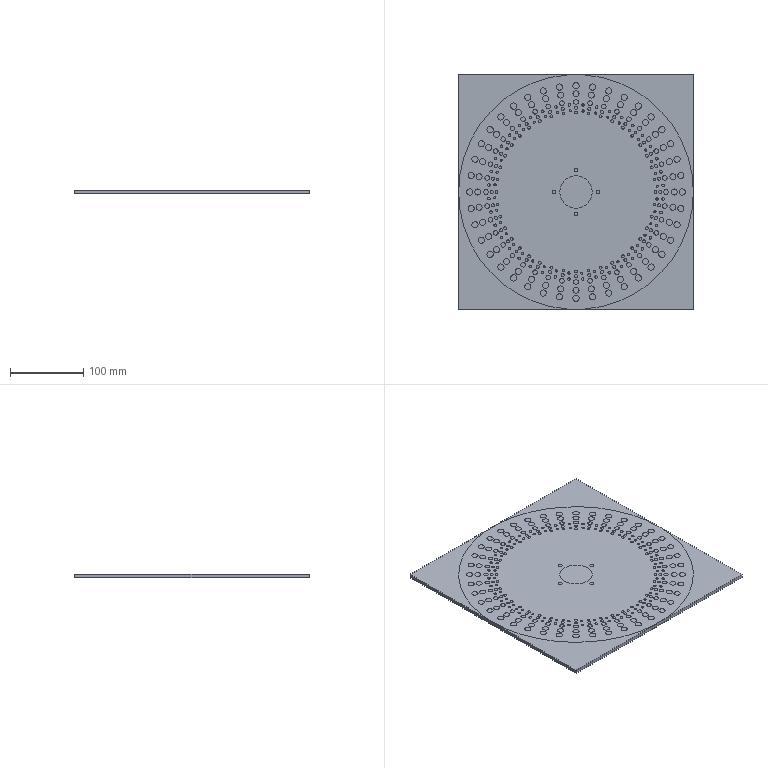NC program | NX | posted with a generic post | part box 320 x 320 x 5 mm
Lines 39666 to 40337 of 63198:
(孔铣精光G41 , TOOL : D6平底刀)
N79324 T08 M6
N79326 /M1
N79328 G54
N79330 G17 G0 G90 X0. Y144.747 S3000 M3
N79332 G43 Z20. H8
N79334 Z1.2
N79336 G94 G1 Z0.2 F400.
N79338 G41 X0.01 Y144.647 D8
N79340 G3 X2.025 Y144.747 R1.01
N79342 X2.025 Y144.747 Z0. I-2.025 J0. F500.
N79344 X2.025 Y144.747 Z-0.2 I-2.025 J0.
N79346 X2.025 Y144.747 Z-0.4 I-2.025 J0.
N79348 X2.025 Y144.747 Z-0.6 I-2.025 J0.
N79350 X2.025 Y144.747 Z-0.8 I-2.025 J0.
N79352 X2.025 Y144.747 Z-1. I-2.025 J0.
N79354 X2.025 Y144.747 Z-1.2 I-2.025 J0.
N79356 X2.025 Y144.747 Z-1.4 I-2.025 J0.
N79358 X2.025 Y144.747 Z-1.6 I-2.025 J0.
N79360 X2.025 Y144.747 Z-1.8 I-2.025 J0.
N79362 X2.025 Y144.747 Z-2. I-2.025 J0.
N79364 X2.025 Y144.747 Z-2.2 I-2.025 J0.
N79366 X2.025 Y144.747 Z-2.4 I-2.025 J0.
N79368 X2.025 Y144.747 Z-2.6 I-2.025 J0.
N79370 X2.025 Y144.747 Z-2.8 I-2.025 J0.
N79372 X2.025 Y144.747 Z-3. I-2.025 J0.
N79374 X2.025 Y144.747 Z-3.2 I-2.025 J0.
N79376 X2.025 Y144.747 Z-3.4 I-2.025 J0.
N79378 X2.025 Y144.747 Z-3.6 I-2.025 J0.
N79380 X2.025 Y144.747 Z-3.8 I-2.025 J0.
N79382 X2.025 Y144.747 Z-4. I-2.025 J0.
N79384 X2.025 Y144.747 Z-4.2 I-2.025 J0.
N79386 X2.025 Y144.747 Z-4.4 I-2.025 J0.
N79388 X2.025 Y144.747 Z-4.6 I-2.025 J0.
N79390 X2.025 Y144.747 Z-4.8 I-2.025 J0.
N79392 X2.025 Y144.747 Z-5. I-2.025 J0.
N79394 X0. Y146.772 R2.025
N79396 X2.025 Y144.747 R-2.025
N79398 X0.01 Y144.846 R1.01
N79400 G40
N79402 G1 X0. Y144.747
N79404 Z-4.8
N79406 G0 Z20.
N79408 X22.643 Y142.965
N79410 Z1.2
N79412 G1 Z0.2 F400.
N79414 G41 X22.653 Y142.865
N79416 G3 X24.668 Y142.965 R1.01
N79418 X24.668 Y142.965 Z0. I-2.025 J0. F500.
N79420 X24.668 Y142.965 Z-0.2 I-2.025 J0.
N79422 X24.668 Y142.965 Z-0.4 I-2.025 J0.
N79424 X24.668 Y142.965 Z-0.6 I-2.025 J0.
N79426 X24.668 Y142.965 Z-0.8 I-2.025 J0.
N79428 X24.668 Y142.965 Z-1. I-2.025 J0.
N79430 X24.668 Y142.965 Z-1.2 I-2.025 J0.
N79432 X24.668 Y142.965 Z-1.4 I-2.025 J0.
N79434 X24.668 Y142.965 Z-1.6 I-2.025 J0.
N79436 X24.668 Y142.965 Z-1.8 I-2.025 J0.
N79438 X24.668 Y142.965 Z-2. I-2.025 J0.
N79440 X24.668 Y142.965 Z-2.2 I-2.025 J0.
N79442 X24.668 Y142.965 Z-2.4 I-2.025 J0.
N79444 X24.668 Y142.965 Z-2.6 I-2.025 J0.
N79446 X24.668 Y142.965 Z-2.8 I-2.025 J0.
N79448 X24.668 Y142.965 Z-3. I-2.025 J0.
N79450 X24.668 Y142.965 Z-3.2 I-2.025 J0.
N79452 X24.668 Y142.965 Z-3.4 I-2.025 J0.
N79454 X24.668 Y142.965 Z-3.6 I-2.025 J0.
N79456 X24.668 Y142.965 Z-3.8 I-2.025 J0.
N79458 X24.668 Y142.965 Z-4. I-2.025 J0.
N79460 X24.668 Y142.965 Z-4.2 I-2.025 J0.
N79462 X24.668 Y142.965 Z-4.4 I-2.025 J0.
N79464 X24.668 Y142.965 Z-4.6 I-2.025 J0.
N79466 X24.668 Y142.965 Z-4.8 I-2.025 J0.
N79468 X24.668 Y142.965 Z-5. I-2.025 J0.
N79470 X22.643 Y144.99 R2.025
N79472 X24.668 Y142.965 R-2.025
N79474 X22.653 Y143.064 R1.01
N79476 G40
N79478 G1 X22.643 Y142.965
N79480 Z-4.8
N79482 G0 Z20.
N79484 X44.729 Y137.662
N79486 Z1.2
N79488 G1 Z0.2 F400.
N79490 G41 X44.739 Y137.563
N79492 G3 X46.754 Y137.662 R1.01
N79494 X46.754 Y137.662 Z0. I-2.025 J0. F500.
N79496 X46.754 Y137.662 Z-0.2 I-2.025 J0.
N79498 X46.754 Y137.662 Z-0.4 I-2.025 J0.
N79500 X46.754 Y137.662 Z-0.6 I-2.025 J0.
N79502 X46.754 Y137.662 Z-0.8 I-2.025 J0.
N79504 X46.754 Y137.662 Z-1. I-2.025 J0.
N79506 X46.754 Y137.662 Z-1.2 I-2.025 J0.
N79508 X46.754 Y137.662 Z-1.4 I-2.025 J0.
N79510 X46.754 Y137.662 Z-1.6 I-2.025 J0.
N79512 X46.754 Y137.662 Z-1.8 I-2.025 J0.
N79514 X46.754 Y137.662 Z-2. I-2.025 J0.
N79516 X46.754 Y137.662 Z-2.2 I-2.025 J0.
N79518 X46.754 Y137.662 Z-2.4 I-2.025 J0.
N79520 X46.754 Y137.662 Z-2.6 I-2.025 J0.
N79522 X46.754 Y137.662 Z-2.8 I-2.025 J0.
N79524 X46.754 Y137.662 Z-3. I-2.025 J0.
N79526 X46.754 Y137.662 Z-3.2 I-2.025 J0.
N79528 X46.754 Y137.662 Z-3.4 I-2.025 J0.
N79530 X46.754 Y137.662 Z-3.6 I-2.025 J0.
N79532 X46.754 Y137.662 Z-3.8 I-2.025 J0.
N79534 X46.754 Y137.662 Z-4. I-2.025 J0.
N79536 X46.754 Y137.662 Z-4.2 I-2.025 J0.
N79538 X46.754 Y137.662 Z-4.4 I-2.025 J0.
N79540 X46.754 Y137.662 Z-4.6 I-2.025 J0.
N79542 X46.754 Y137.662 Z-4.8 I-2.025 J0.
N79544 X46.754 Y137.662 Z-5. I-2.025 J0.
N79546 X44.729 Y139.687 R2.025
N79548 X46.754 Y137.662 R-2.025
N79550 X44.739 Y137.762 R1.01
N79552 G40
N79554 G1 X44.729 Y137.662
N79556 Z-4.8
N79558 G0 Z20.
N79560 X65.714 Y128.97
N79562 Z1.2
N79564 G1 Z0.2 F400.
N79566 G41 X65.724 Y128.871
N79568 G3 X67.739 Y128.97 R1.01
N79570 X67.739 Y128.97 Z0. I-2.025 J0. F500.
N79572 X67.739 Y128.97 Z-0.2 I-2.025 J0.
N79574 X67.739 Y128.97 Z-0.4 I-2.025 J0.
N79576 X67.739 Y128.97 Z-0.6 I-2.025 J0.
N79578 X67.739 Y128.97 Z-0.8 I-2.025 J0.
N79580 X67.739 Y128.97 Z-1. I-2.025 J0.
N79582 X67.739 Y128.97 Z-1.2 I-2.025 J0.
N79584 X67.739 Y128.97 Z-1.4 I-2.025 J0.
N79586 X67.739 Y128.97 Z-1.6 I-2.025 J0.
N79588 X67.739 Y128.97 Z-1.8 I-2.025 J0.
N79590 X67.739 Y128.97 Z-2. I-2.025 J0.
N79592 X67.739 Y128.97 Z-2.2 I-2.025 J0.
N79594 X67.739 Y128.97 Z-2.4 I-2.025 J0.
N79596 X67.739 Y128.97 Z-2.6 I-2.025 J0.
N79598 X67.739 Y128.97 Z-2.8 I-2.025 J0.
N79600 X67.739 Y128.97 Z-3. I-2.025 J0.
N79602 X67.739 Y128.97 Z-3.2 I-2.025 J0.
N79604 X67.739 Y128.97 Z-3.4 I-2.025 J0.
N79606 X67.739 Y128.97 Z-3.6 I-2.025 J0.
N79608 X67.739 Y128.97 Z-3.8 I-2.025 J0.
N79610 X67.739 Y128.97 Z-4. I-2.025 J0.
N79612 X67.739 Y128.97 Z-4.2 I-2.025 J0.
N79614 X67.739 Y128.97 Z-4.4 I-2.025 J0.
N79616 X67.739 Y128.97 Z-4.6 I-2.025 J0.
N79618 X67.739 Y128.97 Z-4.8 I-2.025 J0.
N79620 X67.739 Y128.97 Z-5. I-2.025 J0.
N79622 X65.714 Y130.995 R2.025
N79624 X67.739 Y128.97 R-2.025
N79626 X65.724 Y129.07 R1.01
N79628 G40
N79630 G1 X65.714 Y128.97
N79632 Z-4.8
N79634 G0 Z20.
N79636 X85.08 Y117.103
N79638 Z1.2
N79640 G1 Z0.2 F400.
N79642 G41 X85.09 Y117.003
N79644 G3 X87.105 Y117.103 R1.01
N79646 X87.105 Y117.103 Z0. I-2.025 J0. F500.
N79648 X87.105 Y117.103 Z-0.2 I-2.025 J0.
N79650 X87.105 Y117.103 Z-0.4 I-2.025 J0.
N79652 X87.105 Y117.103 Z-0.6 I-2.025 J0.
N79654 X87.105 Y117.103 Z-0.8 I-2.025 J0.
N79656 X87.105 Y117.103 Z-1. I-2.025 J0.
N79658 X87.105 Y117.103 Z-1.2 I-2.025 J0.
N79660 X87.105 Y117.103 Z-1.4 I-2.025 J0.
N79662 X87.105 Y117.103 Z-1.6 I-2.025 J0.
N79664 X87.105 Y117.103 Z-1.8 I-2.025 J0.
N79666 X87.105 Y117.103 Z-2. I-2.025 J0.
N79668 X87.105 Y117.103 Z-2.2 I-2.025 J0.
N79670 X87.105 Y117.103 Z-2.4 I-2.025 J0.
N79672 X87.105 Y117.103 Z-2.6 I-2.025 J0.
N79674 X87.105 Y117.103 Z-2.8 I-2.025 J0.
N79676 X87.105 Y117.103 Z-3. I-2.025 J0.
N79678 X87.105 Y117.103 Z-3.2 I-2.025 J0.
N79680 X87.105 Y117.103 Z-3.4 I-2.025 J0.
N79682 X87.105 Y117.103 Z-3.6 I-2.025 J0.
N79684 X87.105 Y117.103 Z-3.8 I-2.025 J0.
N79686 X87.105 Y117.103 Z-4. I-2.025 J0.
N79688 X87.105 Y117.103 Z-4.2 I-2.025 J0.
N79690 X87.105 Y117.103 Z-4.4 I-2.025 J0.
N79692 X87.105 Y117.103 Z-4.6 I-2.025 J0.
N79694 X87.105 Y117.103 Z-4.8 I-2.025 J0.
N79696 X87.105 Y117.103 Z-5. I-2.025 J0.
N79698 X85.08 Y119.128 R2.025
N79700 X87.105 Y117.103 R-2.025
N79702 X85.09 Y117.202 R1.01
N79704 G40
N79706 G1 X85.08 Y117.103
N79708 Z-4.8
N79710 G0 Z20.
N79712 X102.351 Y102.351
N79714 Z1.2
N79716 G1 Z0.2 F400.
N79718 G41 X102.361 Y102.252
N79720 G3 X104.376 Y102.351 R1.01
N79722 X104.376 Y102.351 Z0. I-2.025 J0. F500.
N79724 X104.376 Y102.351 Z-0.2 I-2.025 J0.
N79726 X104.376 Y102.351 Z-0.4 I-2.025 J0.
N79728 X104.376 Y102.351 Z-0.6 I-2.025 J0.
N79730 X104.376 Y102.351 Z-0.8 I-2.025 J0.
N79732 X104.376 Y102.351 Z-1. I-2.025 J0.
N79734 X104.376 Y102.351 Z-1.2 I-2.025 J0.
N79736 X104.376 Y102.351 Z-1.4 I-2.025 J0.
N79738 X104.376 Y102.351 Z-1.6 I-2.025 J0.
N79740 X104.376 Y102.351 Z-1.8 I-2.025 J0.
N79742 X104.376 Y102.351 Z-2. I-2.025 J0.
N79744 X104.376 Y102.351 Z-2.2 I-2.025 J0.
N79746 X104.376 Y102.351 Z-2.4 I-2.025 J0.
N79748 X104.376 Y102.351 Z-2.6 I-2.025 J0.
N79750 X104.376 Y102.351 Z-2.8 I-2.025 J0.
N79752 X104.376 Y102.351 Z-3. I-2.025 J0.
N79754 X104.376 Y102.351 Z-3.2 I-2.025 J0.
N79756 X104.376 Y102.351 Z-3.4 I-2.025 J0.
N79758 X104.376 Y102.351 Z-3.6 I-2.025 J0.
N79760 X104.376 Y102.351 Z-3.8 I-2.025 J0.
N79762 X104.376 Y102.351 Z-4. I-2.025 J0.
N79764 X104.376 Y102.351 Z-4.2 I-2.025 J0.
N79766 X104.376 Y102.351 Z-4.4 I-2.025 J0.
N79768 X104.376 Y102.351 Z-4.6 I-2.025 J0.
N79770 X104.376 Y102.351 Z-4.8 I-2.025 J0.
N79772 X104.376 Y102.351 Z-5. I-2.025 J0.
N79774 X102.351 Y104.376 R2.025
N79776 X104.376 Y102.351 R-2.025
N79778 X102.361 Y102.451 R1.01
N79780 G40
N79782 G1 X102.351 Y102.351
N79784 Z-4.8
N79786 G0 Z20.
N79788 X117.103 Y85.08
N79790 Z1.2
N79792 G1 Z0.2 F400.
N79794 G41 X117.112 Y84.981
N79796 G3 X119.128 Y85.08 R1.01
N79798 X119.128 Y85.08 Z0. I-2.025 J0. F500.
N79800 X119.128 Y85.08 Z-0.2 I-2.025 J0.
N79802 X119.128 Y85.08 Z-0.4 I-2.025 J0.
N79804 X119.128 Y85.08 Z-0.6 I-2.025 J0.
N79806 X119.128 Y85.08 Z-0.8 I-2.025 J0.
N79808 X119.128 Y85.08 Z-1. I-2.025 J0.
N79810 X119.128 Y85.08 Z-1.2 I-2.025 J0.
N79812 X119.128 Y85.08 Z-1.4 I-2.025 J0.
N79814 X119.128 Y85.08 Z-1.6 I-2.025 J0.
N79816 X119.128 Y85.08 Z-1.8 I-2.025 J0.
N79818 X119.128 Y85.08 Z-2. I-2.025 J0.
N79820 X119.128 Y85.08 Z-2.2 I-2.025 J0.
N79822 X119.128 Y85.08 Z-2.4 I-2.025 J0.
N79824 X119.128 Y85.08 Z-2.6 I-2.025 J0.
N79826 X119.128 Y85.08 Z-2.8 I-2.025 J0.
N79828 X119.128 Y85.08 Z-3. I-2.025 J0.
N79830 X119.128 Y85.08 Z-3.2 I-2.025 J0.
N79832 X119.128 Y85.08 Z-3.4 I-2.025 J0.
N79834 X119.128 Y85.08 Z-3.6 I-2.025 J0.
N79836 X119.128 Y85.08 Z-3.8 I-2.025 J0.
N79838 X119.128 Y85.08 Z-4. I-2.025 J0.
N79840 X119.128 Y85.08 Z-4.2 I-2.025 J0.
N79842 X119.128 Y85.08 Z-4.4 I-2.025 J0.
N79844 X119.128 Y85.08 Z-4.6 I-2.025 J0.
N79846 X119.128 Y85.08 Z-4.8 I-2.025 J0.
N79848 X119.128 Y85.08 Z-5. I-2.025 J0.
N79850 X117.103 Y87.105 R2.025
N79852 X119.128 Y85.08 R-2.025
N79854 X117.112 Y85.18 R1.01
N79856 G40
N79858 G1 X117.103 Y85.08
N79860 Z-4.8
N79862 G0 Z20.
N79864 X128.97 Y65.714
N79866 Z1.2
N79868 G1 Z0.2 F400.
N79870 G41 X128.98 Y65.614
N79872 G3 X130.995 Y65.714 R1.01
N79874 X130.995 Y65.714 Z0. I-2.025 J0. F500.
N79876 X130.995 Y65.714 Z-0.2 I-2.025 J0.
N79878 X130.995 Y65.714 Z-0.4 I-2.025 J0.
N79880 X130.995 Y65.714 Z-0.6 I-2.025 J0.
N79882 X130.995 Y65.714 Z-0.8 I-2.025 J0.
N79884 X130.995 Y65.714 Z-1. I-2.025 J0.
N79886 X130.995 Y65.714 Z-1.2 I-2.025 J0.
N79888 X130.995 Y65.714 Z-1.4 I-2.025 J0.
N79890 X130.995 Y65.714 Z-1.6 I-2.025 J0.
N79892 X130.995 Y65.714 Z-1.8 I-2.025 J0.
N79894 X130.995 Y65.714 Z-2. I-2.025 J0.
N79896 X130.995 Y65.714 Z-2.2 I-2.025 J0.
N79898 X130.995 Y65.714 Z-2.4 I-2.025 J0.
N79900 X130.995 Y65.714 Z-2.6 I-2.025 J0.
N79902 X130.995 Y65.714 Z-2.8 I-2.025 J0.
N79904 X130.995 Y65.714 Z-3. I-2.025 J0.
N79906 X130.995 Y65.714 Z-3.2 I-2.025 J0.
N79908 X130.995 Y65.714 Z-3.4 I-2.025 J0.
N79910 X130.995 Y65.714 Z-3.6 I-2.025 J0.
N79912 X130.995 Y65.714 Z-3.8 I-2.025 J0.
N79914 X130.995 Y65.714 Z-4. I-2.025 J0.
N79916 X130.995 Y65.714 Z-4.2 I-2.025 J0.
N79918 X130.995 Y65.714 Z-4.4 I-2.025 J0.
N79920 X130.995 Y65.714 Z-4.6 I-2.025 J0.
N79922 X130.995 Y65.714 Z-4.8 I-2.025 J0.
N79924 X130.995 Y65.714 Z-5. I-2.025 J0.
N79926 X128.97 Y67.739 R2.025
N79928 X130.995 Y65.714 R-2.025
N79930 X128.98 Y65.813 R1.01
N79932 G40
N79934 G1 X128.97 Y65.714
N79936 Z-4.8
N79938 G0 Z20.
N79940 X137.662 Y44.729
N79942 Z1.2
N79944 G1 Z0.2 F400.
N79946 G41 X137.672 Y44.63
N79948 G3 X139.687 Y44.729 R1.01
N79950 X139.687 Y44.729 Z0. I-2.025 J0. F500.
N79952 X139.687 Y44.729 Z-0.2 I-2.025 J0.
N79954 X139.687 Y44.729 Z-0.4 I-2.025 J0.
N79956 X139.687 Y44.729 Z-0.6 I-2.025 J0.
N79958 X139.687 Y44.729 Z-0.8 I-2.025 J0.
N79960 X139.687 Y44.729 Z-1. I-2.025 J0.
N79962 X139.687 Y44.729 Z-1.2 I-2.025 J0.
N79964 X139.687 Y44.729 Z-1.4 I-2.025 J0.
N79966 X139.687 Y44.729 Z-1.6 I-2.025 J0.
N79968 X139.687 Y44.729 Z-1.8 I-2.025 J0.
N79970 X139.687 Y44.729 Z-2. I-2.025 J0.
N79972 X139.687 Y44.729 Z-2.2 I-2.025 J0.
N79974 X139.687 Y44.729 Z-2.4 I-2.025 J0.
N79976 X139.687 Y44.729 Z-2.6 I-2.025 J0.
N79978 X139.687 Y44.729 Z-2.8 I-2.025 J0.
N79980 X139.687 Y44.729 Z-3. I-2.025 J0.
N79982 X139.687 Y44.729 Z-3.2 I-2.025 J0.
N79984 X139.687 Y44.729 Z-3.4 I-2.025 J0.
N79986 X139.687 Y44.729 Z-3.6 I-2.025 J0.
N79988 X139.687 Y44.729 Z-3.8 I-2.025 J0.
N79990 X139.687 Y44.729 Z-4. I-2.025 J0.
N79992 X139.687 Y44.729 Z-4.2 I-2.025 J0.
N79994 X139.687 Y44.729 Z-4.4 I-2.025 J0.
N79996 X139.687 Y44.729 Z-4.6 I-2.025 J0.
N79998 X139.687 Y44.729 Z-4.8 I-2.025 J0.
N80000 X139.687 Y44.729 Z-5. I-2.025 J0.
N80002 X137.662 Y46.754 R2.025
N80004 X139.687 Y44.729 R-2.025
N80006 X137.672 Y44.829 R1.01
N80008 G40
N80010 G1 X137.662 Y44.729
N80012 Z-4.8
N80014 G0 Z20.
N80016 X142.965 Y22.643
N80018 Z1.2
N80020 G1 Z0.2 F400.
N80022 G41 X142.975 Y22.544
N80024 G3 X144.99 Y22.643 R1.01
N80026 X144.99 Y22.643 Z0. I-2.025 J0. F500.
N80028 X144.99 Y22.643 Z-0.2 I-2.025 J0.
N80030 X144.99 Y22.643 Z-0.4 I-2.025 J0.
N80032 X144.99 Y22.643 Z-0.6 I-2.025 J0.
N80034 X144.99 Y22.643 Z-0.8 I-2.025 J0.
N80036 X144.99 Y22.643 Z-1. I-2.025 J0.
N80038 X144.99 Y22.643 Z-1.2 I-2.025 J0.
N80040 X144.99 Y22.643 Z-1.4 I-2.025 J0.
N80042 X144.99 Y22.643 Z-1.6 I-2.025 J0.
N80044 X144.99 Y22.643 Z-1.8 I-2.025 J0.
N80046 X144.99 Y22.643 Z-2. I-2.025 J0.
N80048 X144.99 Y22.643 Z-2.2 I-2.025 J0.
N80050 X144.99 Y22.643 Z-2.4 I-2.025 J0.
N80052 X144.99 Y22.643 Z-2.6 I-2.025 J0.
N80054 X144.99 Y22.643 Z-2.8 I-2.025 J0.
N80056 X144.99 Y22.643 Z-3. I-2.025 J0.
N80058 X144.99 Y22.643 Z-3.2 I-2.025 J0.
N80060 X144.99 Y22.643 Z-3.4 I-2.025 J0.
N80062 X144.99 Y22.643 Z-3.6 I-2.025 J0.
N80064 X144.99 Y22.643 Z-3.8 I-2.025 J0.
N80066 X144.99 Y22.643 Z-4. I-2.025 J0.
N80068 X144.99 Y22.643 Z-4.2 I-2.025 J0.
N80070 X144.99 Y22.643 Z-4.4 I-2.025 J0.
N80072 X144.99 Y22.643 Z-4.6 I-2.025 J0.
N80074 X144.99 Y22.643 Z-4.8 I-2.025 J0.
N80076 X144.99 Y22.643 Z-5. I-2.025 J0.
N80078 X142.965 Y24.668 R2.025
N80080 X144.99 Y22.643 R-2.025
N80082 X142.975 Y22.743 R1.01
N80084 G40
N80086 G1 X142.965 Y22.643
N80088 Z-4.8
N80090 G0 Z20.
N80092 X144.747 Y0.
N80094 Z1.2
N80096 G1 Z0.2 F400.
N80098 G41 X144.757 Y-0.1
N80100 G3 X146.772 Y0. R1.01
N80102 X146.772 Y0. Z0. I-2.025 J0. F500.
N80104 X146.772 Y0. Z-0.2 I-2.025 J0.
N80106 X146.772 Y0. Z-0.4 I-2.025 J0.
N80108 X146.772 Y0. Z-0.6 I-2.025 J0.
N80110 X146.772 Y0. Z-0.8 I-2.025 J0.
N80112 X146.772 Y0. Z-1. I-2.025 J0.
N80114 X146.772 Y0. Z-1.2 I-2.025 J0.
N80116 X146.772 Y0. Z-1.4 I-2.025 J0.
N80118 X146.772 Y0. Z-1.6 I-2.025 J0.
N80120 X146.772 Y0. Z-1.8 I-2.025 J0.
N80122 X146.772 Y0. Z-2. I-2.025 J0.
N80124 X146.772 Y0. Z-2.2 I-2.025 J0.
N80126 X146.772 Y0. Z-2.4 I-2.025 J0.
N80128 X146.772 Y0. Z-2.6 I-2.025 J0.
N80130 X146.772 Y0. Z-2.8 I-2.025 J0.
N80132 X146.772 Y0. Z-3. I-2.025 J0.
N80134 X146.772 Y0. Z-3.2 I-2.025 J0.
N80136 X146.772 Y0. Z-3.4 I-2.025 J0.
N80138 X146.772 Y0. Z-3.6 I-2.025 J0.
N80140 X146.772 Y0. Z-3.8 I-2.025 J0.
N80142 X146.772 Y0. Z-4. I-2.025 J0.
N80144 X146.772 Y0. Z-4.2 I-2.025 J0.
N80146 X146.772 Y0. Z-4.4 I-2.025 J0.
N80148 X146.772 Y0. Z-4.6 I-2.025 J0.
N80150 X146.772 Y0. Z-4.8 I-2.025 J0.
N80152 X146.772 Y0. Z-5. I-2.025 J0.
N80154 X144.747 Y2.025 R2.025
N80156 X146.772 Y0. R-2.025
N80158 X144.757 Y0.1 R1.01
N80160 G40
N80162 G1 X144.747 Y0.
N80164 Z-4.8
N80166 G0 Z20.
N80168 X142.965 Y-22.643
N80170 Z1.2
N80172 G1 Z0.2 F400.
N80174 G41 X142.975 Y-22.743
N80176 G3 X144.99 Y-22.643 R1.01
N80178 X144.99 Y-22.643 Z0. I-2.025 J0. F500.
N80180 X144.99 Y-22.643 Z-0.2 I-2.025 J0.
N80182 X144.99 Y-22.643 Z-0.4 I-2.025 J0.
N80184 X144.99 Y-22.643 Z-0.6 I-2.025 J0.
N80186 X144.99 Y-22.643 Z-0.8 I-2.025 J0.
N80188 X144.99 Y-22.643 Z-1. I-2.025 J0.
N80190 X144.99 Y-22.643 Z-1.2 I-2.025 J0.
N80192 X144.99 Y-22.643 Z-1.4 I-2.025 J0.
N80194 X144.99 Y-22.643 Z-1.6 I-2.025 J0.
N80196 X144.99 Y-22.643 Z-1.8 I-2.025 J0.
N80198 X144.99 Y-22.643 Z-2. I-2.025 J0.
N80200 X144.99 Y-22.643 Z-2.2 I-2.025 J0.
N80202 X144.99 Y-22.643 Z-2.4 I-2.025 J0.
N80204 X144.99 Y-22.643 Z-2.6 I-2.025 J0.
N80206 X144.99 Y-22.643 Z-2.8 I-2.025 J0.
N80208 X144.99 Y-22.643 Z-3. I-2.025 J0.
N80210 X144.99 Y-22.643 Z-3.2 I-2.025 J0.
N80212 X144.99 Y-22.643 Z-3.4 I-2.025 J0.
N80214 X144.99 Y-22.643 Z-3.6 I-2.025 J0.
N80216 X144.99 Y-22.643 Z-3.8 I-2.025 J0.
N80218 X144.99 Y-22.643 Z-4. I-2.025 J0.
N80220 X144.99 Y-22.643 Z-4.2 I-2.025 J0.
N80222 X144.99 Y-22.643 Z-4.4 I-2.025 J0.
N80224 X144.99 Y-22.643 Z-4.6 I-2.025 J0.
N80226 X144.99 Y-22.643 Z-4.8 I-2.025 J0.
N80228 X144.99 Y-22.643 Z-5. I-2.025 J0.
N80230 X142.965 Y-20.618 R2.025
N80232 X144.99 Y-22.643 R-2.025
N80234 X142.975 Y-22.544 R1.01
N80236 G40
N80238 G1 X142.965 Y-22.643
N80240 Z-4.8
N80242 G0 Z20.
N80244 X137.662 Y-44.729
N80246 Z1.2
N80248 G1 Z0.2 F400.
N80250 G41 X137.672 Y-44.829
N80252 G3 X139.687 Y-44.729 R1.01
N80254 X139.687 Y-44.729 Z0. I-2.025 J0. F500.
N80256 X139.687 Y-44.729 Z-0.2 I-2.025 J0.
N80258 X139.687 Y-44.729 Z-0.4 I-2.025 J0.
N80260 X139.687 Y-44.729 Z-0.6 I-2.025 J0.
N80262 X139.687 Y-44.729 Z-0.8 I-2.025 J0.
N80264 X139.687 Y-44.729 Z-1. I-2.025 J0.
N80266 X139.687 Y-44.729 Z-1.2 I-2.025 J0.
N80268 X139.687 Y-44.729 Z-1.4 I-2.025 J0.
N80270 X139.687 Y-44.729 Z-1.6 I-2.025 J0.
N80272 X139.687 Y-44.729 Z-1.8 I-2.025 J0.
N80274 X139.687 Y-44.729 Z-2. I-2.025 J0.
N80276 X139.687 Y-44.729 Z-2.2 I-2.025 J0.
N80278 X139.687 Y-44.729 Z-2.4 I-2.025 J0.
N80280 X139.687 Y-44.729 Z-2.6 I-2.025 J0.
N80282 X139.687 Y-44.729 Z-2.8 I-2.025 J0.
N80284 X139.687 Y-44.729 Z-3. I-2.025 J0.
N80286 X139.687 Y-44.729 Z-3.2 I-2.025 J0.
N80288 X139.687 Y-44.729 Z-3.4 I-2.025 J0.
N80290 X139.687 Y-44.729 Z-3.6 I-2.025 J0.
N80292 X139.687 Y-44.729 Z-3.8 I-2.025 J0.
N80294 X139.687 Y-44.729 Z-4. I-2.025 J0.
N80296 X139.687 Y-44.729 Z-4.2 I-2.025 J0.
N80298 X139.687 Y-44.729 Z-4.4 I-2.025 J0.
N80300 X139.687 Y-44.729 Z-4.6 I-2.025 J0.
N80302 X139.687 Y-44.729 Z-4.8 I-2.025 J0.
N80304 X139.687 Y-44.729 Z-5. I-2.025 J0.
N80306 X137.662 Y-42.704 R2.025
N80308 X139.687 Y-44.729 R-2.025
N80310 X137.672 Y-44.63 R1.01
N80312 G40
N80314 G1 X137.662 Y-44.729
N80316 Z-4.8
N80318 G0 Z20.
N80320 X128.97 Y-65.714
N80322 Z1.2
N80324 G1 Z0.2 F400.
N80326 G41 X128.98 Y-65.813
N80328 G3 X130.995 Y-65.714 R1.01
N80330 X130.995 Y-65.714 Z0. I-2.025 J0. F500.
N80332 X130.995 Y-65.714 Z-0.2 I-2.025 J0.
N80334 X130.995 Y-65.714 Z-0.4 I-2.025 J0.
N80336 X130.995 Y-65.714 Z-0.6 I-2.025 J0.
N80338 X130.995 Y-65.714 Z-0.8 I-2.025 J0.
N80340 X130.995 Y-65.714 Z-1. I-2.025 J0.
N80342 X130.995 Y-65.714 Z-1.2 I-2.025 J0.
N80344 X130.995 Y-65.714 Z-1.4 I-2.025 J0.
N80346 X130.995 Y-65.714 Z-1.6 I-2.025 J0.
N80348 X130.995 Y-65.714 Z-1.8 I-2.025 J0.
N80350 X130.995 Y-65.714 Z-2. I-2.025 J0.
N80352 X130.995 Y-65.714 Z-2.2 I-2.025 J0.
N80354 X130.995 Y-65.714 Z-2.4 I-2.025 J0.
N80356 X130.995 Y-65.714 Z-2.6 I-2.025 J0.
N80358 X130.995 Y-65.714 Z-2.8 I-2.025 J0.
N80360 X130.995 Y-65.714 Z-3. I-2.025 J0.
N80362 X130.995 Y-65.714 Z-3.2 I-2.025 J0.
N80364 X130.995 Y-65.714 Z-3.4 I-2.025 J0.
N80366 X130.995 Y-65.714 Z-3.6 I-2.025 J0.
N80368 X130.995 Y-65.714 Z-3.8 I-2.025 J0.
N80370 X130.995 Y-65.714 Z-4. I-2.025 J0.
N80372 X130.995 Y-65.714 Z-4.2 I-2.025 J0.
N80374 X130.995 Y-65.714 Z-4.4 I-2.025 J0.
N80376 X130.995 Y-65.714 Z-4.6 I-2.025 J0.
N80378 X130.995 Y-65.714 Z-4.8 I-2.025 J0.
N80380 X130.995 Y-65.714 Z-5. I-2.025 J0.
N80382 X128.97 Y-63.689 R2.025
N80384 X130.995 Y-65.714 R-2.025
N80386 X128.98 Y-65.614 R1.01
N80388 G40
N80390 G1 X128.97 Y-65.714
N80392 Z-4.8
N80394 G0 Z20.
N80396 X117.103 Y-85.08
N80398 Z1.2
N80400 G1 Z0.2 F400.
N80402 G41 X117.112 Y-85.18
N80404 G3 X119.128 Y-85.08 R1.01
N80406 X119.128 Y-85.08 Z0. I-2.025 J0. F500.
N80408 X119.128 Y-85.08 Z-0.2 I-2.025 J0.
N80410 X119.128 Y-85.08 Z-0.4 I-2.025 J0.
N80412 X119.128 Y-85.08 Z-0.6 I-2.025 J0.
N80414 X119.128 Y-85.08 Z-0.8 I-2.025 J0.
N80416 X119.128 Y-85.08 Z-1. I-2.025 J0.
N80418 X119.128 Y-85.08 Z-1.2 I-2.025 J0.
N80420 X119.128 Y-85.08 Z-1.4 I-2.025 J0.
N80422 X119.128 Y-85.08 Z-1.6 I-2.025 J0.
N80424 X119.128 Y-85.08 Z-1.8 I-2.025 J0.
N80426 X119.128 Y-85.08 Z-2. I-2.025 J0.
N80428 X119.128 Y-85.08 Z-2.2 I-2.025 J0.
N80430 X119.128 Y-85.08 Z-2.4 I-2.025 J0.
N80432 X119.128 Y-85.08 Z-2.6 I-2.025 J0.
N80434 X119.128 Y-85.08 Z-2.8 I-2.025 J0.
N80436 X119.128 Y-85.08 Z-3. I-2.025 J0.
N80438 X119.128 Y-85.08 Z-3.2 I-2.025 J0.
N80440 X119.128 Y-85.08 Z-3.4 I-2.025 J0.
N80442 X119.128 Y-85.08 Z-3.6 I-2.025 J0.
N80444 X119.128 Y-85.08 Z-3.8 I-2.025 J0.
N80446 X119.128 Y-85.08 Z-4. I-2.025 J0.
N80448 X119.128 Y-85.08 Z-4.2 I-2.025 J0.
N80450 X119.128 Y-85.08 Z-4.4 I-2.025 J0.
N80452 X119.128 Y-85.08 Z-4.6 I-2.025 J0.
N80454 X119.128 Y-85.08 Z-4.8 I-2.025 J0.
N80456 X119.128 Y-85.08 Z-5. I-2.025 J0.
N80458 X117.103 Y-83.055 R2.025
N80460 X119.128 Y-85.08 R-2.025
N80462 X117.112 Y-84.981 R1.01
N80464 G40
N80466 G1 X117.103 Y-85.08
N80468 Z-4.8
N80470 G0 Z20.
N80472 X102.351 Y-102.351
N80474 Z1.2
N80476 G1 Z0.2 F400.
N80478 G41 X102.361 Y-102.451
N80480 G3 X104.376 Y-102.351 R1.01
N80482 X104.376 Y-102.351 Z0. I-2.025 J0. F500.
N80484 X104.376 Y-102.351 Z-0.2 I-2.025 J0.
N80486 X104.376 Y-102.351 Z-0.4 I-2.025 J0.
N80488 X104.376 Y-102.351 Z-0.6 I-2.025 J0.
N80490 X104.376 Y-102.351 Z-0.8 I-2.025 J0.
N80492 X104.376 Y-102.351 Z-1. I-2.025 J0.
N80494 X104.376 Y-102.351 Z-1.2 I-2.025 J0.
N80496 X104.376 Y-102.351 Z-1.4 I-2.025 J0.
N80498 X104.376 Y-102.351 Z-1.6 I-2.025 J0.
N80500 X104.376 Y-102.351 Z-1.8 I-2.025 J0.
N80502 X104.376 Y-102.351 Z-2. I-2.025 J0.
N80504 X104.376 Y-102.351 Z-2.2 I-2.025 J0.
N80506 X104.376 Y-102.351 Z-2.4 I-2.025 J0.
N80508 X104.376 Y-102.351 Z-2.6 I-2.025 J0.
N80510 X104.376 Y-102.351 Z-2.8 I-2.025 J0.
N80512 X104.376 Y-102.351 Z-3. I-2.025 J0.
N80514 X104.376 Y-102.351 Z-3.2 I-2.025 J0.
N80516 X104.376 Y-102.351 Z-3.4 I-2.025 J0.
N80518 X104.376 Y-102.351 Z-3.6 I-2.025 J0.
N80520 X104.376 Y-102.351 Z-3.8 I-2.025 J0.
N80522 X104.376 Y-102.351 Z-4. I-2.025 J0.
N80524 X104.376 Y-102.351 Z-4.2 I-2.025 J0.
N80526 X104.376 Y-102.351 Z-4.4 I-2.025 J0.
N80528 X104.376 Y-102.351 Z-4.6 I-2.025 J0.
N80530 X104.376 Y-102.351 Z-4.8 I-2.025 J0.
N80532 X104.376 Y-102.351 Z-5. I-2.025 J0.
N80534 X102.351 Y-100.326 R2.025
N80536 X104.376 Y-102.351 R-2.025
N80538 X102.361 Y-102.252 R1.01
N80540 G40
N80542 G1 X102.351 Y-102.351
N80544 Z-4.8
N80546 G0 Z20.
N80548 X85.08 Y-117.103
N80550 Z1.2
N80552 G1 Z0.2 F400.
N80554 G41 X85.09 Y-117.202
N80556 G3 X87.105 Y-117.103 R1.01
N80558 X87.105 Y-117.103 Z0. I-2.025 J0. F500.
N80560 X87.105 Y-117.103 Z-0.2 I-2.025 J0.
N80562 X87.105 Y-117.103 Z-0.4 I-2.025 J0.
N80564 X87.105 Y-117.103 Z-0.6 I-2.025 J0.
N80566 X87.105 Y-117.103 Z-0.8 I-2.025 J0.
N80568 X87.105 Y-117.103 Z-1. I-2.025 J0.
N80570 X87.105 Y-117.103 Z-1.2 I-2.025 J0.
N80572 X87.105 Y-117.103 Z-1.4 I-2.025 J0.
N80574 X87.105 Y-117.103 Z-1.6 I-2.025 J0.
N80576 X87.105 Y-117.103 Z-1.8 I-2.025 J0.
N80578 X87.105 Y-117.103 Z-2. I-2.025 J0.
N80580 X87.105 Y-117.103 Z-2.2 I-2.025 J0.
N80582 X87.105 Y-117.103 Z-2.4 I-2.025 J0.
N80584 X87.105 Y-117.103 Z-2.6 I-2.025 J0.
N80586 X87.105 Y-117.103 Z-2.8 I-2.025 J0.
N80588 X87.105 Y-117.103 Z-3. I-2.025 J0.
N80590 X87.105 Y-117.103 Z-3.2 I-2.025 J0.
N80592 X87.105 Y-117.103 Z-3.4 I-2.025 J0.
N80594 X87.105 Y-117.103 Z-3.6 I-2.025 J0.
N80596 X87.105 Y-117.103 Z-3.8 I-2.025 J0.
N80598 X87.105 Y-117.103 Z-4. I-2.025 J0.
N80600 X87.105 Y-117.103 Z-4.2 I-2.025 J0.
N80602 X87.105 Y-117.103 Z-4.4 I-2.025 J0.
N80604 X87.105 Y-117.103 Z-4.6 I-2.025 J0.
N80606 X87.105 Y-117.103 Z-4.8 I-2.025 J0.
N80608 X87.105 Y-117.103 Z-5. I-2.025 J0.
N80610 X85.08 Y-115.078 R2.025
N80612 X87.105 Y-117.103 R-2.025
N80614 X85.09 Y-117.003 R1.01
N80616 G40
N80618 G1 X85.08 Y-117.103
N80620 Z-4.8
N80622 G0 Z20.
N80624 X65.714 Y-128.97
N80626 Z1.2
N80628 G1 Z0.2 F400.
N80630 G41 X65.724 Y-129.07
N80632 G3 X67.739 Y-128.97 R1.01
N80634 X67.739 Y-128.97 Z0. I-2.025 J0. F500.
N80636 X67.739 Y-128.97 Z-0.2 I-2.025 J0.
N80638 X67.739 Y-128.97 Z-0.4 I-2.025 J0.
N80640 X67.739 Y-128.97 Z-0.6 I-2.025 J0.
N80642 X67.739 Y-128.97 Z-0.8 I-2.025 J0.
N80644 X67.739 Y-128.97 Z-1. I-2.025 J0.
N80646 X67.739 Y-128.97 Z-1.2 I-2.025 J0.
N80648 X67.739 Y-128.97 Z-1.4 I-2.025 J0.
N80650 X67.739 Y-128.97 Z-1.6 I-2.025 J0.
N80652 X67.739 Y-128.97 Z-1.8 I-2.025 J0.
N80654 X67.739 Y-128.97 Z-2. I-2.025 J0.
N80656 X67.739 Y-128.97 Z-2.2 I-2.025 J0.
N80658 X67.739 Y-128.97 Z-2.4 I-2.025 J0.
N80660 X67.739 Y-128.97 Z-2.6 I-2.025 J0.